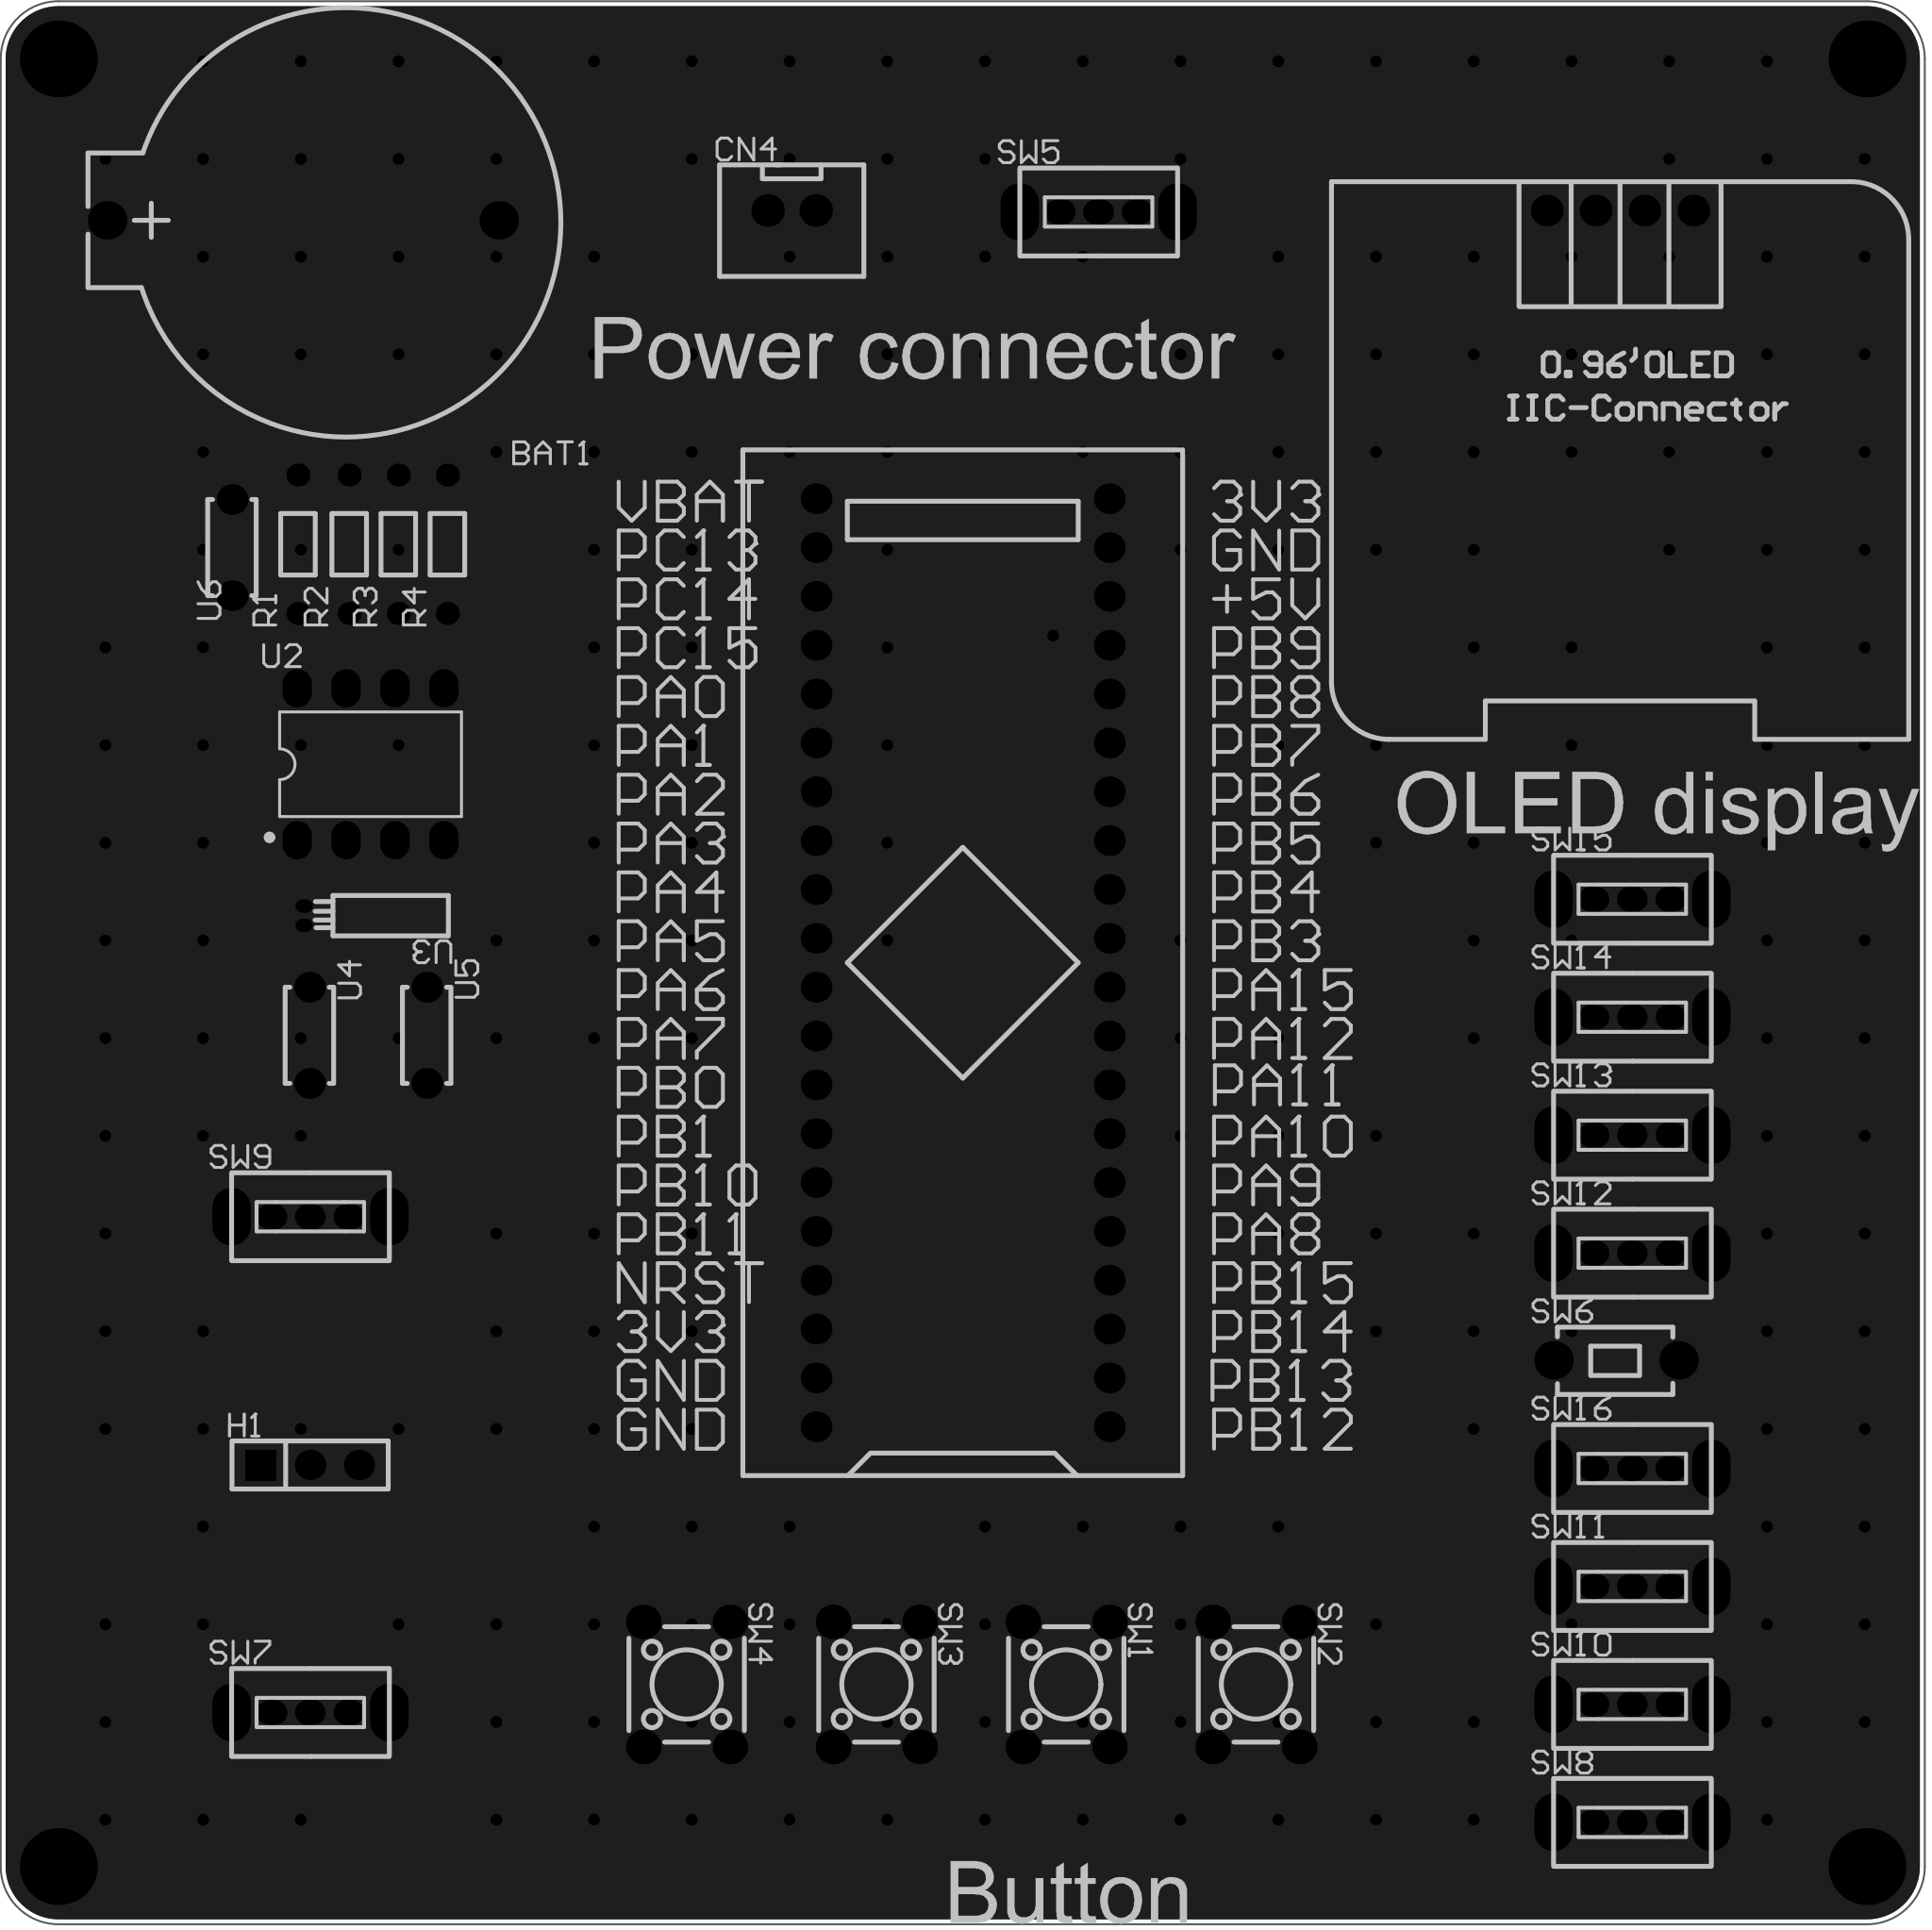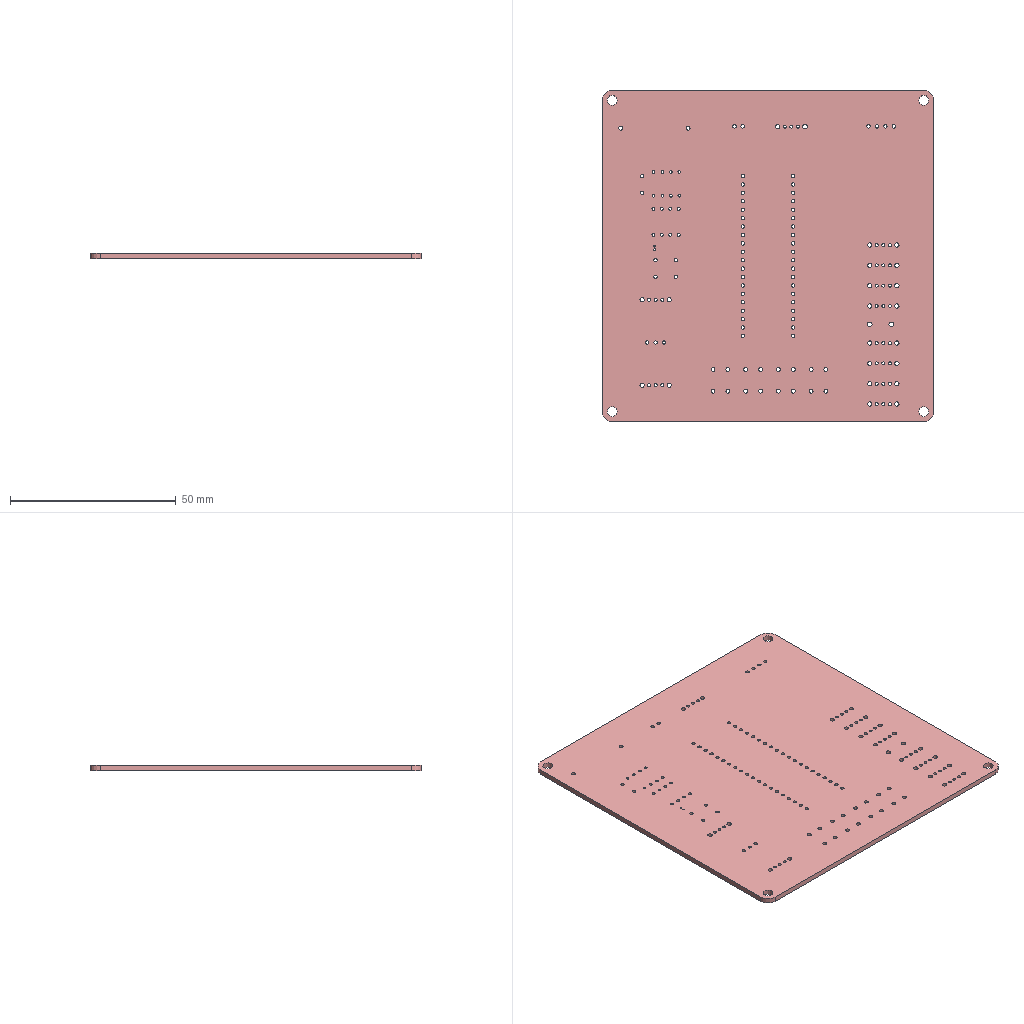Circuit board layout | Altium Designer | box 100 x 100 x 1.6 mm
Layer stack:
# Altium Designer layer stack of  (unit mm; dielectric type: 0 none, 1 core, 2 prepreg, 3 surface material)
index,name,kind,layer,copper_thickness_mm,dielectric_type,dielectric_thickness_mm,dielectric_material,dielectric_constant
0,Top Paste Mask Layer,other,,,,,,
1,Top Silkscreen Layer,other,,,,,,
2,Top Solder Mask Layer,dielectric,,,3,0.01,,3.3
3,Top Layer,copper,Top Layer,0.035,,,,
4,Dielectric1,dielectric,,,3,1.51,FR4,4.5
5,Bottom Layer,copper,Bottom Layer,0.035,,,,
6,Bottom Solder Mask Layer,dielectric,,,3,0.01,,3.3
7,Bottom Silkscreen Layer,other,,,,,,
8,Bottom Paste Mask Layer,other,,,,,,
# drill layer pairs: low layer,high layer
drill_pair,Top Layer,Bottom Layer
Part placement:
Designator,Comment,Layer,Footprint,Center-X(mm),Center-Y(mm),Rotation
U1,STM32F103C8T6-Card,TopLayer,CONN-TH_L53.3-W22.9_STM32F103C8T6-CARD,141.351,130.937,90
OLED1,,TopLayer,0.96OLED_4P,175.514,170.053,0
SW1,,TopLayer,SW-TH_4P-L6.0-W6.0-P4.50-LS6.5,146.727,93.408,270
SW2,,TopLayer,SW-TH_4P-L6.0-W6.0-P4.50-LS6.5,156.591,93.408,270
SW3,,TopLayer,SW-TH_4P-L6.0-W6.0-P4.50-LS6.5,136.864,93.408,270
SW4,,TopLayer,SW-TH_4P-L6.0-W6.0-P4.50-LS6.5,127,93.408,270
CN4,XH2.54*2P_through-hole,TopLayer,CONN-TH_2P-P2.50-XH2.54-2P,132.461,170.053,0
SW5,,TopLayer,拨动开关,148.417,169.978,0
BAT1,CR2032-2-1,TopLayer,BAT-TH_CR2032-2-1,107.061,169.545,180
H1,,TopLayer,HDR-TH_3P-P2.54-V-F,107.431,104.82,0
R1,10kΩ,TopLayer,Res_1/8W,106.8,152.699,90
SW6,,TopLayer,Key_TH_3.5x6x4.3,175.307,110.264,0
SW7,,TopLayer,拨动开关,107.45,91.948,0
SW8,,TopLayer,拨动开关,176.157,86.233,0
SW9,,TopLayer,拨动开关,107.45,117.729,0
SW10,,TopLayer,拨动开关,176.157,92.368,0
SW11,,TopLayer,拨动开关,176.157,98.502,0
SW12,,TopLayer,拨动开关,176.157,115.835,0
SW13,,TopLayer,拨动开关,176.157,121.969,0
SW14,,TopLayer,拨动开关,176.157,128.104,0
SW15,,TopLayer,拨动开关,176.157,134.239,0
SW16,,TopLayer,拨动开关,176.157,104.637,0
U2,DS1302N(LX),TopLayer,PDIP-8_L9.3-W6.4-P2.54-LS7.9-BL-1,110.572,141.26,0
U3,32.768kHz,TopLayer,CRYSTAL-TH_BD2.1-P0.70-D0.3,107.117,133.385,180
U4,30pF,TopLayer,CAP-TH_L5.0-W2.5-P5.00-D1.0,107.403,127.163,270
U5,30pF,TopLayer,CAP-TH_L5.0-W2.5-P5.00-D1.0,113.499,127.163,270
U6,1nF,TopLayer,CAP-TH_L5.0-W2.5-P5.00-D1.0,103.378,152.527,270
R2,10kΩ,TopLayer,Res_1/8W,109.462,152.699,90
R3,10kΩ,TopLayer,Res_1/8W,112.015,152.699,90
R4,10kΩ,TopLayer,Res_1/8W,114.567,152.699,90
Pad and via stacks:
# Altium Designer via and pad stacks of  (unit mm). Each distinct definition once, with the count of objects using it.
# via: kind,start_layer,end_layer,hole_mm,diameter_mm,mode(0 simple;1 top-mid-bottom;2 full stack),diameter_per_layer,count,example_net
# pad: kind,layer,hole_mm,hole_type(0 round;1 square;2 slot),plating,top_size,top_shape(1 round;2 rect;3 octagon;9 rounded rect),mid_size,bottom_size,mode,footprint,size_per_layer,count,example
pad,Multi-Layer,3,0,plated,4x4,1,4x4,4x4,0,,,4,1
pad,Multi-Layer,1,0,plated,1.6x1.6,1,1.6x1.6,1.6x1.6,0,CONN-TH_L53.3-W22.9_STM32F103C8T6-CARD,,40,U1.1
pad,Multi-Layer,1,0,plated,1.65x1.65,1,1.65x1.65,1.65x1.65,0,0.96OLED_4P,,4,OLED1.4
pad,Multi-Layer,1.2,0,plated,1.8x1.8,1,1.8x1.8,1.8x1.8,0,SW-TH_4P-L6.0-W6.0-P4.50-LS6.5,,16,SW1.1
pad,Multi-Layer,1.05,0,plated,1.7x1.7,1,1.7x1.7,1.7x1.7,0,CONN-TH_2P-P2.50-XH2.54-2P,,2,CN4.2
pad,Multi-Layer,0.8992,0,plated,1.6x1.3,1,1.6x1.3,1.6x1.3,0,\u00B2\u00A6\u00B6\u00AF\u00BF\u00AA\u00B9\u00D8,,33,SW5.1
pad,Multi-Layer,1.3,0,plated,3x1.999,1,3x1.999,3x1.999,0,\u00B2\u00A6\u00B6\u00AF\u00BF\u00AA\u00B9\u00D8,,22,SW5.4
pad,Multi-Layer,1.2,0,plated,2x2,1,2x2,2x2,0,BAT-TH_CR2032-2-1,,2,BAT1.2
pad,Multi-Layer,1.02,0,plated,1.575x1.575,1,1.575x1.575,1.575x1.575,0,HDR-TH_3P-P2.54-V-F,,2,H1.3
pad,Multi-Layer,1.02,0,plated,1.575x1.575,2,1.575x1.575,1.575x1.575,0,HDR-TH_3P-P2.54-V-F,,1,H1.1
pad,Multi-Layer,0.8001,0,plated,1.199x1.199,1,1.199x1.199,1.199x1.199,0,Res_1/8W,,8,R1.1
pad,Multi-Layer,1.399,0,plated,1.999x1.999,1,1.999x1.999,1.999x1.999,0,Key_TH_3.5x6x4.3,,2,SW6.A
pad,Multi-Layer,0.9,0,plated,1.524x2,1,1.524x2,1.524x2,0,PDIP-8_L9.3-W6.4-P2.54-LS7.9-BL-1,,8,U2.1
pad,Multi-Layer,0.5,0,plated,0.9x0.7,1,0.9x0.7,0.9x0.7,0,CRYSTAL-TH_BD2.1-P0.70-D0.3,,2,U3.1
pad,Multi-Layer,1,0,plated,1.6x1.6,1,1.6x1.6,1.6x1.6,0,CAP-TH_L5.0-W2.5-P5.00-D1.0,,6,U4.1
via,Top Layer,Bottom Layer,0.3048,0.61,0,,235,VCC
Copper pours:
name,layer,net,type(0 solid;1 hatched;2 none)
Bottom Layer-GND,Bottom Layer,GND,0
Top Layer-GND,Top Layer,GND,0